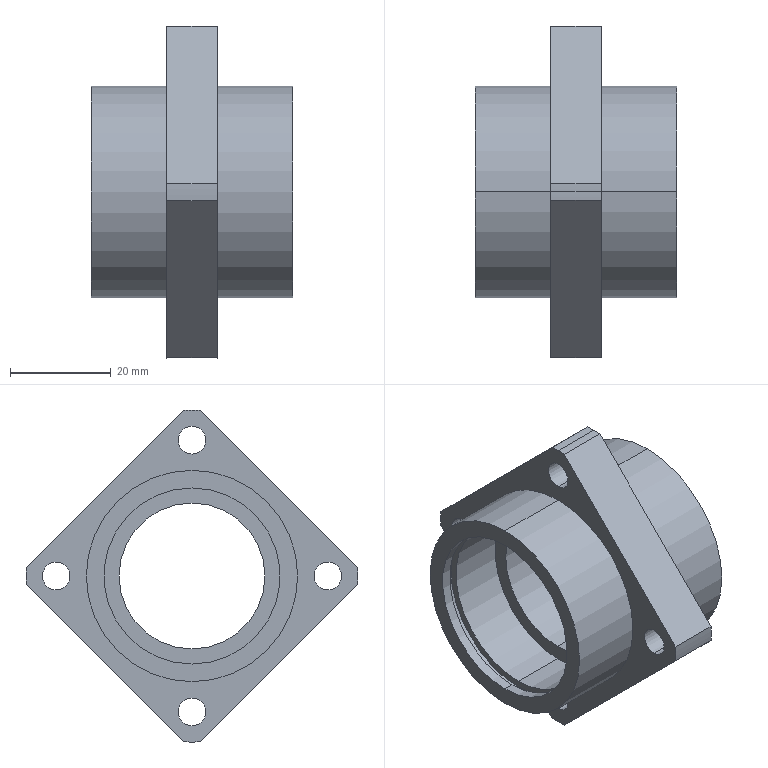Part | STEP file | _housing_bgfszb6202-40-15 | 1 solid | 57 faces | box 40 x 66 x 66 mm | volume 27673 mm3 | cylinder 39 | plane 18 | commonest cylinder face diameters 5.5 x8 9.5 x8 35 x8 66 x5 37.8 x4 42 x4